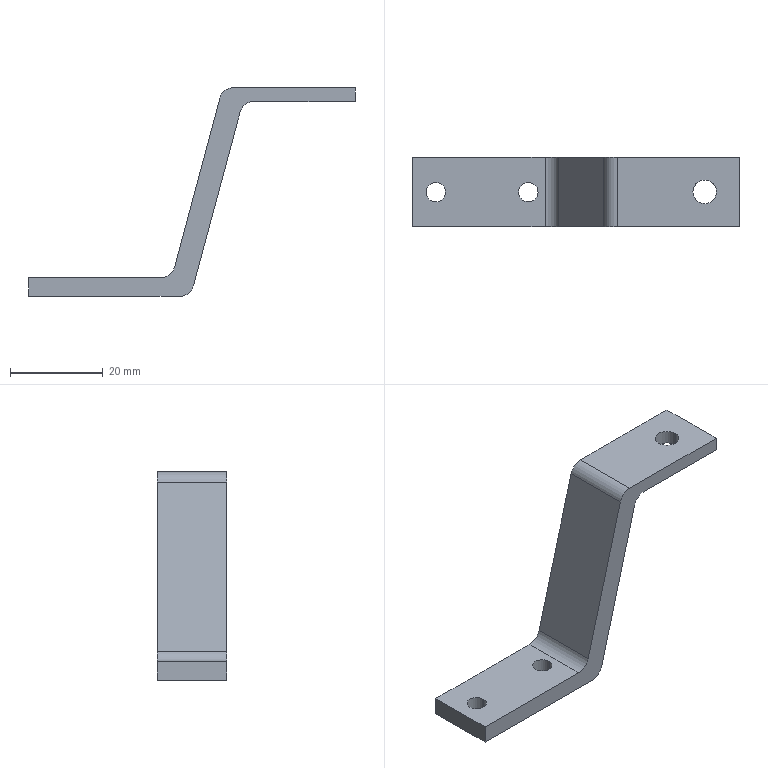Part | SolidWorks | features Extrusion 1, Fillet 1, ICE 1 | 1 solid | 20 faces | box 70.55 x 15 x 45 mm | volume 6219 mm3 | cylinder 10 | plane 10 | commonest cylinder face diameters 4.2 x4 6 x4 5.1 x2
STEP:
#1=CARTESIAN_POINT('',(27.1,7.5,4.));
#2=VERTEX_POINT('',#1);
#3=CARTESIAN_POINT('',(22.9,7.5,4.));
#4=VERTEX_POINT('',#3);
#5=CARTESIAN_POINT('',(25.,7.5,4.));
#6=DIRECTION('',(0.,0.,-1.));
#7=DIRECTION('',(-1.,0.,0.));
#8=AXIS2_PLACEMENT_3D('',#5,#6,#7);
#9=CIRCLE('',#8,2.1);
#10=EDGE_CURVE('',#2,#4,#9,.T.);
#11=ORIENTED_EDGE('',*,*,#10,.F.);
#12=CARTESIAN_POINT('',(27.1,7.5,0.));
#13=VERTEX_POINT('',#12);
#14=CARTESIAN_POINT('',(27.1,7.5,45.));
#15=DIRECTION('',(0.,0.,-1.));
#16=VECTOR('',#15,1000.);
#17=LINE('',#14,#16);
#18=EDGE_CURVE('',#2,#13,#17,.T.);
#19=ORIENTED_EDGE('',*,*,#18,.T.);
#20=CARTESIAN_POINT('',(22.9,7.5,0.));
#21=VERTEX_POINT('',#20);
#22=CARTESIAN_POINT('',(25.,7.5,0.));
#23=DIRECTION('',(0.,0.,-1.));
#24=DIRECTION('',(-1.,0.,0.));
#25=AXIS2_PLACEMENT_3D('',#22,#23,#24);
#26=CIRCLE('',#25,2.1);
#27=EDGE_CURVE('',#13,#21,#26,.T.);
#28=ORIENTED_EDGE('',*,*,#27,.T.);
#29=CARTESIAN_POINT('',(22.9,7.5,45.));
#30=DIRECTION('',(0.,0.,-1.));
#31=VECTOR('',#30,1000.);
#32=LINE('',#29,#31);
#33=EDGE_CURVE('',#4,#21,#32,.T.);
#34=ORIENTED_EDGE('',*,*,#33,.F.);
#35=EDGE_LOOP('',(#11,#19,#28,#34));
#36=FACE_OUTER_BOUND('',#35,.T.);
#37=CARTESIAN_POINT('',(25.,7.5,45.));
#38=DIRECTION('',(0.,0.,-1.));
#39=DIRECTION('',(-1.,0.,0.));
#40=AXIS2_PLACEMENT_3D('',#37,#38,#39);
#41=CYLINDRICAL_SURFACE('',#40,2.1);
#42=ADVANCED_FACE('',(#36),#41,.F.);
#43=CARTESIAN_POINT('',(7.1,7.5,4.));
#44=VERTEX_POINT('',#43);
#45=CARTESIAN_POINT('',(2.9,7.5,4.));
#46=VERTEX_POINT('',#45);
#47=CARTESIAN_POINT('',(5.,7.5,4.));
#48=DIRECTION('',(0.,0.,-1.));
#49=DIRECTION('',(-1.,0.,0.));
#50=AXIS2_PLACEMENT_3D('',#47,#48,#49);
#51=CIRCLE('',#50,2.1);
#52=EDGE_CURVE('',#44,#46,#51,.T.);
#53=ORIENTED_EDGE('',*,*,#52,.F.);
#54=CARTESIAN_POINT('',(7.1,7.5,0.));
#55=VERTEX_POINT('',#54);
#56=CARTESIAN_POINT('',(7.1,7.5,45.));
#57=DIRECTION('',(0.,0.,-1.));
#58=VECTOR('',#57,1000.);
#59=LINE('',#56,#58);
#60=EDGE_CURVE('',#44,#55,#59,.T.);
#61=ORIENTED_EDGE('',*,*,#60,.T.);
#62=CARTESIAN_POINT('',(2.9,7.5,0.));
#63=VERTEX_POINT('',#62);
#64=CARTESIAN_POINT('',(5.,7.5,0.));
#65=DIRECTION('',(0.,0.,-1.));
#66=DIRECTION('',(-1.,0.,0.));
#67=AXIS2_PLACEMENT_3D('',#64,#65,#66);
#68=CIRCLE('',#67,2.1);
#69=EDGE_CURVE('',#55,#63,#68,.T.);
#70=ORIENTED_EDGE('',*,*,#69,.T.);
#71=CARTESIAN_POINT('',(2.9,7.5,45.));
#72=DIRECTION('',(0.,0.,-1.));
#73=VECTOR('',#72,1000.);
#74=LINE('',#71,#73);
#75=EDGE_CURVE('',#46,#63,#74,.T.);
#76=ORIENTED_EDGE('',*,*,#75,.F.);
#77=EDGE_LOOP('',(#53,#61,#70,#76));
#78=FACE_OUTER_BOUND('',#77,.T.);
#79=CARTESIAN_POINT('',(5.,7.5,45.));
#80=DIRECTION('',(0.,0.,-1.));
#81=DIRECTION('',(-1.,0.,0.));
#82=AXIS2_PLACEMENT_3D('',#79,#80,#81);
#83=CYLINDRICAL_SURFACE('',#82,2.1);
#84=ADVANCED_FACE('',(#78),#83,.F.);
#85=CARTESIAN_POINT('',(65.6,7.5,45.));
#86=VERTEX_POINT('',#85);
#87=CARTESIAN_POINT('',(60.5,7.5,45.));
#88=VERTEX_POINT('',#87);
#89=CARTESIAN_POINT('',(63.05,7.5,45.));
#90=DIRECTION('',(0.,0.,-1.));
#91=DIRECTION('',(-1.,0.,0.));
#92=AXIS2_PLACEMENT_3D('',#89,#90,#91);
#93=CIRCLE('',#92,2.55);
#94=EDGE_CURVE('',#86,#88,#93,.T.);
#95=ORIENTED_EDGE('',*,*,#94,.F.);
#96=CARTESIAN_POINT('',(65.6,7.5,42.));
#97=VERTEX_POINT('',#96);
#98=CARTESIAN_POINT('',(65.6,7.5,45.));
#99=DIRECTION('',(0.,0.,-1.));
#100=VECTOR('',#99,1000.);
#101=LINE('',#98,#100);
#102=EDGE_CURVE('',#86,#97,#101,.T.);
#103=ORIENTED_EDGE('',*,*,#102,.T.);
#104=CARTESIAN_POINT('',(60.5,7.5,42.));
#105=VERTEX_POINT('',#104);
#106=CARTESIAN_POINT('',(63.05,7.5,42.));
#107=DIRECTION('',(0.,0.,1.));
#108=DIRECTION('',(1.,0.,0.));
#109=AXIS2_PLACEMENT_3D('',#106,#107,#108);
#110=CIRCLE('',#109,2.55);
#111=EDGE_CURVE('',#105,#97,#110,.T.);
#112=ORIENTED_EDGE('',*,*,#111,.F.);
#113=CARTESIAN_POINT('',(60.5,7.5,45.));
#114=DIRECTION('',(0.,0.,-1.));
#115=VECTOR('',#114,1000.);
#116=LINE('',#113,#115);
#117=EDGE_CURVE('',#88,#105,#116,.T.);
#118=ORIENTED_EDGE('',*,*,#117,.F.);
#119=EDGE_LOOP('',(#95,#103,#112,#118));
#120=FACE_OUTER_BOUND('',#119,.T.);
#121=CARTESIAN_POINT('',(63.05,7.5,45.));
#122=DIRECTION('',(0.,0.,-1.));
#123=DIRECTION('',(-1.,0.,0.));
#124=AXIS2_PLACEMENT_3D('',#121,#122,#123);
#125=CYLINDRICAL_SURFACE('',#124,2.55);
#126=ADVANCED_FACE('',(#120),#125,.F.);
#127=CARTESIAN_POINT('',(25.,7.5,0.));
#128=DIRECTION('',(0.,0.,-1.));
#129=DIRECTION('',(-1.,0.,0.));
#130=AXIS2_PLACEMENT_3D('',#127,#128,#129);
#131=CIRCLE('',#130,2.1);
#132=EDGE_CURVE('',#21,#13,#131,.T.);
#133=ORIENTED_EDGE('',*,*,#132,.F.);
#134=ORIENTED_EDGE('',*,*,#27,.F.);
#135=EDGE_LOOP('',(#133,#134));
#136=FACE_BOUND('',#135,.T.);
#137=CARTESIAN_POINT('',(5.,7.5,0.));
#138=DIRECTION('',(0.,0.,-1.));
#139=DIRECTION('',(-1.,0.,0.));
#140=AXIS2_PLACEMENT_3D('',#137,#138,#139);
#141=CIRCLE('',#140,2.1);
#142=EDGE_CURVE('',#63,#55,#141,.T.);
#143=ORIENTED_EDGE('',*,*,#142,.F.);
#144=ORIENTED_EDGE('',*,*,#69,.F.);
#145=EDGE_LOOP('',(#143,#144));
#146=FACE_BOUND('',#145,.T.);
#147=CARTESIAN_POINT('',(32.698,15.,0.));
#148=VERTEX_POINT('',#147);
#149=CARTESIAN_POINT('',(0.,15.,0.));
#150=VERTEX_POINT('',#149);
#151=CARTESIAN_POINT('',(35.,15.,0.));
#152=DIRECTION('',(-1.,0.,0.));
#153=VECTOR('',#152,1000.);
#154=LINE('',#151,#153);
#155=EDGE_CURVE('',#148,#150,#154,.T.);
#156=ORIENTED_EDGE('',*,*,#155,.F.);
#157=CARTESIAN_POINT('',(32.698,0.,0.));
#158=VERTEX_POINT('',#157);
#159=CARTESIAN_POINT('',(32.698,15.,0.));
#160=DIRECTION('',(0.,-1.,0.));
#161=VECTOR('',#160,1000.);
#162=LINE('',#159,#161);
#163=EDGE_CURVE('',#148,#158,#162,.T.);
#164=ORIENTED_EDGE('',*,*,#163,.T.);
#165=CARTESIAN_POINT('',(0.,0.,0.));
#166=VERTEX_POINT('',#165);
#167=CARTESIAN_POINT('',(35.,0.,0.));
#168=DIRECTION('',(-1.,0.,0.));
#169=VECTOR('',#168,1000.);
#170=LINE('',#167,#169);
#171=EDGE_CURVE('',#158,#166,#170,.T.);
#172=ORIENTED_EDGE('',*,*,#171,.T.);
#173=CARTESIAN_POINT('',(0.,15.,0.));
#174=DIRECTION('',(0.,-1.,0.));
#175=VECTOR('',#174,1000.);
#176=LINE('',#173,#175);
#177=EDGE_CURVE('',#150,#166,#176,.T.);
#178=ORIENTED_EDGE('',*,*,#177,.F.);
#179=EDGE_LOOP('',(#156,#164,#172,#178));
#180=FACE_OUTER_BOUND('',#179,.T.);
#181=CARTESIAN_POINT('',(35.,15.,0.));
#182=DIRECTION('',(0.,0.,1.));
#183=DIRECTION('',(1.,0.,0.));
#184=AXIS2_PLACEMENT_3D('',#181,#182,#183);
#185=PLANE('',#184);
#186=ADVANCED_FACE('',(#136,#146,#180),#185,.F.);
#187=CARTESIAN_POINT('',(0.,0.,4.));
#188=VERTEX_POINT('',#187);
#189=CARTESIAN_POINT('',(0.,0.,0.));
#190=DIRECTION('',(0.,0.,1.));
#191=VECTOR('',#190,1000.);
#192=LINE('',#189,#191);
#193=EDGE_CURVE('',#166,#188,#192,.T.);
#194=ORIENTED_EDGE('',*,*,#193,.T.);
#195=CARTESIAN_POINT('',(0.,15.,4.));
#196=VERTEX_POINT('',#195);
#197=CARTESIAN_POINT('',(0.,15.,4.));
#198=DIRECTION('',(0.,-1.,0.));
#199=VECTOR('',#198,1000.);
#200=LINE('',#197,#199);
#201=EDGE_CURVE('',#196,#188,#200,.T.);
#202=ORIENTED_EDGE('',*,*,#201,.F.);
#203=CARTESIAN_POINT('',(0.,15.,0.));
#204=DIRECTION('',(0.,0.,1.));
#205=VECTOR('',#204,1000.);
#206=LINE('',#203,#205);
#207=EDGE_CURVE('',#150,#196,#206,.T.);
#208=ORIENTED_EDGE('',*,*,#207,.F.);
#209=ORIENTED_EDGE('',*,*,#177,.T.);
#210=EDGE_LOOP('',(#194,#202,#208,#209));
#211=FACE_OUTER_BOUND('',#210,.T.);
#212=CARTESIAN_POINT('',(0.,15.,0.));
#213=DIRECTION('',(1.,0.,0.));
#214=DIRECTION('',(0.,0.,-1.));
#215=AXIS2_PLACEMENT_3D('',#212,#213,#214);
#216=PLANE('',#215);
#217=ADVANCED_FACE('',(#211),#216,.F.);
#218=CARTESIAN_POINT('',(25.,7.5,4.));
#219=DIRECTION('',(0.,0.,-1.));
#220=DIRECTION('',(-1.,0.,0.));
#221=AXIS2_PLACEMENT_3D('',#218,#219,#220);
#222=CIRCLE('',#221,2.1);
#223=EDGE_CURVE('',#4,#2,#222,.T.);
#224=ORIENTED_EDGE('',*,*,#223,.T.);
#225=ORIENTED_EDGE('',*,*,#10,.T.);
#226=EDGE_LOOP('',(#224,#225));
#227=FACE_BOUND('',#226,.T.);
#228=CARTESIAN_POINT('',(5.,7.5,4.));
#229=DIRECTION('',(0.,0.,-1.));
#230=DIRECTION('',(-1.,0.,0.));
#231=AXIS2_PLACEMENT_3D('',#228,#229,#230);
#232=CIRCLE('',#231,2.1);
#233=EDGE_CURVE('',#46,#44,#232,.T.);
#234=ORIENTED_EDGE('',*,*,#233,.T.);
#235=ORIENTED_EDGE('',*,*,#52,.T.);
#236=EDGE_LOOP('',(#234,#235));
#237=FACE_BOUND('',#236,.T.);
#238=CARTESIAN_POINT('',(28.593,0.,4.));
#239=VERTEX_POINT('',#238);
#240=CARTESIAN_POINT('',(0.,0.,4.));
#241=DIRECTION('',(1.,0.,0.));
#242=VECTOR('',#241,1000.);
#243=LINE('',#240,#242);
#244=EDGE_CURVE('',#188,#239,#243,.T.);
#245=ORIENTED_EDGE('',*,*,#244,.T.);
#246=CARTESIAN_POINT('',(28.593,15.,4.));
#247=VERTEX_POINT('',#246);
#248=CARTESIAN_POINT('',(28.593,15.,4.));
#249=DIRECTION('',(0.,1.,0.));
#250=VECTOR('',#249,1000.);
#251=LINE('',#248,#250);
#252=EDGE_CURVE('',#239,#247,#251,.T.);
#253=ORIENTED_EDGE('',*,*,#252,.T.);
#254=CARTESIAN_POINT('',(0.,15.,4.));
#255=DIRECTION('',(1.,0.,0.));
#256=VECTOR('',#255,1000.);
#257=LINE('',#254,#256);
#258=EDGE_CURVE('',#196,#247,#257,.T.);
#259=ORIENTED_EDGE('',*,*,#258,.F.);
#260=ORIENTED_EDGE('',*,*,#201,.T.);
#261=EDGE_LOOP('',(#245,#253,#259,#260));
#262=FACE_OUTER_BOUND('',#261,.T.);
#263=CARTESIAN_POINT('',(0.,15.,4.));
#264=DIRECTION('',(0.,0.,-1.));
#265=DIRECTION('',(-1.,0.,0.));
#266=AXIS2_PLACEMENT_3D('',#263,#264,#265);
#267=PLANE('',#266);
#268=ADVANCED_FACE('',(#227,#237,#262),#267,.F.);
#269=CARTESIAN_POINT('',(31.491,0.,6.224));
#270=VERTEX_POINT('',#269);
#271=CARTESIAN_POINT('',(41.286,0.,42.776));
#272=VERTEX_POINT('',#271);
#273=CARTESIAN_POINT('',(30.895,0.,4.));
#274=DIRECTION('',(0.2588,0.,0.9659));
#275=VECTOR('',#274,1000.);
#276=LINE('',#273,#275);
#277=EDGE_CURVE('',#270,#272,#276,.T.);
#278=ORIENTED_EDGE('',*,*,#277,.T.);
#279=CARTESIAN_POINT('',(41.286,15.,42.776));
#280=VERTEX_POINT('',#279);
#281=CARTESIAN_POINT('',(41.286,15.,42.776));
#282=DIRECTION('',(0.,1.,0.));
#283=VECTOR('',#282,1000.);
#284=LINE('',#281,#283);
#285=EDGE_CURVE('',#272,#280,#284,.T.);
#286=ORIENTED_EDGE('',*,*,#285,.T.);
#287=CARTESIAN_POINT('',(31.491,15.,6.224));
#288=VERTEX_POINT('',#287);
#289=CARTESIAN_POINT('',(30.895,15.,4.));
#290=DIRECTION('',(0.2588,0.,0.9659));
#291=VECTOR('',#290,1000.);
#292=LINE('',#289,#291);
#293=EDGE_CURVE('',#288,#280,#292,.T.);
#294=ORIENTED_EDGE('',*,*,#293,.F.);
#295=CARTESIAN_POINT('',(31.491,0.,6.224));
#296=DIRECTION('',(0.,-1.,0.));
#297=VECTOR('',#296,1000.);
#298=LINE('',#295,#297);
#299=EDGE_CURVE('',#288,#270,#298,.T.);
#300=ORIENTED_EDGE('',*,*,#299,.T.);
#301=EDGE_LOOP('',(#278,#286,#294,#300));
#302=FACE_OUTER_BOUND('',#301,.T.);
#303=CARTESIAN_POINT('',(30.895,15.,4.));
#304=DIRECTION('',(0.9659,0.,-0.2588));
#305=DIRECTION('',(-0.2588,0.,-0.9659));
#306=AXIS2_PLACEMENT_3D('',#303,#304,#305);
#307=PLANE('',#306);
#308=ADVANCED_FACE('',(#302),#307,.F.);
#309=CARTESIAN_POINT('',(63.05,7.5,45.));
#310=DIRECTION('',(0.,0.,-1.));
#311=DIRECTION('',(-1.,0.,0.));
#312=AXIS2_PLACEMENT_3D('',#309,#310,#311);
#313=CIRCLE('',#312,2.55);
#314=EDGE_CURVE('',#88,#86,#313,.T.);
#315=ORIENTED_EDGE('',*,*,#314,.T.);
#316=ORIENTED_EDGE('',*,*,#94,.T.);
#317=EDGE_LOOP('',(#315,#316));
#318=FACE_BOUND('',#317,.T.);
#319=CARTESIAN_POINT('',(44.183,15.,45.));
#320=VERTEX_POINT('',#319);
#321=CARTESIAN_POINT('',(70.55,15.,45.));
#322=VERTEX_POINT('',#321);
#323=CARTESIAN_POINT('',(41.881,15.,45.));
#324=DIRECTION('',(1.,0.,0.));
#325=VECTOR('',#324,1000.);
#326=LINE('',#323,#325);
#327=EDGE_CURVE('',#320,#322,#326,.T.);
#328=ORIENTED_EDGE('',*,*,#327,.F.);
#329=CARTESIAN_POINT('',(44.183,0.,45.));
#330=VERTEX_POINT('',#329);
#331=CARTESIAN_POINT('',(44.183,15.,45.));
#332=DIRECTION('',(0.,-1.,0.));
#333=VECTOR('',#332,1000.);
#334=LINE('',#331,#333);
#335=EDGE_CURVE('',#320,#330,#334,.T.);
#336=ORIENTED_EDGE('',*,*,#335,.T.);
#337=CARTESIAN_POINT('',(70.55,0.,45.));
#338=VERTEX_POINT('',#337);
#339=CARTESIAN_POINT('',(41.881,0.,45.));
#340=DIRECTION('',(1.,0.,0.));
#341=VECTOR('',#340,1000.);
#342=LINE('',#339,#341);
#343=EDGE_CURVE('',#330,#338,#342,.T.);
#344=ORIENTED_EDGE('',*,*,#343,.T.);
#345=CARTESIAN_POINT('',(70.55,15.,45.));
#346=DIRECTION('',(0.,-1.,0.));
#347=VECTOR('',#346,1000.);
#348=LINE('',#345,#347);
#349=EDGE_CURVE('',#322,#338,#348,.T.);
#350=ORIENTED_EDGE('',*,*,#349,.F.);
#351=EDGE_LOOP('',(#328,#336,#344,#350));
#352=FACE_OUTER_BOUND('',#351,.T.);
#353=CARTESIAN_POINT('',(41.881,15.,45.));
#354=DIRECTION('',(0.,0.,-1.));
#355=DIRECTION('',(-1.,0.,0.));
#356=AXIS2_PLACEMENT_3D('',#353,#354,#355);
#357=PLANE('',#356);
#358=ADVANCED_FACE('',(#318,#352),#357,.F.);
#359=CARTESIAN_POINT('',(70.55,0.,42.));
#360=VERTEX_POINT('',#359);
#361=CARTESIAN_POINT('',(70.55,0.,45.));
#362=DIRECTION('',(0.,0.,-1.));
#363=VECTOR('',#362,1000.);
#364=LINE('',#361,#363);
#365=EDGE_CURVE('',#338,#360,#364,.T.);
#366=ORIENTED_EDGE('',*,*,#365,.T.);
#367=CARTESIAN_POINT('',(70.55,15.,42.));
#368=VERTEX_POINT('',#367);
#369=CARTESIAN_POINT('',(70.55,15.,42.));
#370=DIRECTION('',(0.,-1.,0.));
#371=VECTOR('',#370,1000.);
#372=LINE('',#369,#371);
#373=EDGE_CURVE('',#368,#360,#372,.T.);
#374=ORIENTED_EDGE('',*,*,#373,.F.);
#375=CARTESIAN_POINT('',(70.55,15.,45.));
#376=DIRECTION('',(0.,0.,-1.));
#377=VECTOR('',#376,1000.);
#378=LINE('',#375,#377);
#379=EDGE_CURVE('',#322,#368,#378,.T.);
#380=ORIENTED_EDGE('',*,*,#379,.F.);
#381=ORIENTED_EDGE('',*,*,#349,.T.);
#382=EDGE_LOOP('',(#366,#374,#380,#381));
#383=FACE_OUTER_BOUND('',#382,.T.);
#384=CARTESIAN_POINT('',(70.55,15.,45.));
#385=DIRECTION('',(-1.,0.,0.));
#386=DIRECTION('',(0.,0.,1.));
#387=AXIS2_PLACEMENT_3D('',#384,#385,#386);
#388=PLANE('',#387);
#389=ADVANCED_FACE('',(#383),#388,.F.);
#390=ORIENTED_EDGE('',*,*,#111,.T.);
#391=CARTESIAN_POINT('',(63.05,7.5,42.));
#392=DIRECTION('',(0.,0.,1.));
#393=DIRECTION('',(1.,0.,0.));
#394=AXIS2_PLACEMENT_3D('',#391,#392,#393);
#395=CIRCLE('',#394,2.55);
#396=EDGE_CURVE('',#97,#105,#395,.T.);
#397=ORIENTED_EDGE('',*,*,#396,.T.);
#398=EDGE_LOOP('',(#390,#397));
#399=FACE_BOUND('',#398,.T.);
#400=CARTESIAN_POINT('',(48.556,0.,42.));
#401=VERTEX_POINT('',#400);
#402=CARTESIAN_POINT('',(70.55,0.,42.));
#403=DIRECTION('',(-1.,0.,0.));
#404=VECTOR('',#403,1000.);
#405=LINE('',#402,#404);
#406=EDGE_CURVE('',#360,#401,#405,.T.);
#407=ORIENTED_EDGE('',*,*,#406,.T.);
#408=CARTESIAN_POINT('',(48.556,15.,42.));
#409=VERTEX_POINT('',#408);
#410=CARTESIAN_POINT('',(48.556,15.,42.));
#411=DIRECTION('',(0.,1.,0.));
#412=VECTOR('',#411,1000.);
#413=LINE('',#410,#412);
#414=EDGE_CURVE('',#401,#409,#413,.T.);
#415=ORIENTED_EDGE('',*,*,#414,.T.);
#416=CARTESIAN_POINT('',(70.55,15.,42.));
#417=DIRECTION('',(-1.,0.,0.));
#418=VECTOR('',#417,1000.);
#419=LINE('',#416,#418);
#420=EDGE_CURVE('',#368,#409,#419,.T.);
#421=ORIENTED_EDGE('',*,*,#420,.F.);
#422=ORIENTED_EDGE('',*,*,#373,.T.);
#423=EDGE_LOOP('',(#407,#415,#421,#422));
#424=FACE_OUTER_BOUND('',#423,.T.);
#425=CARTESIAN_POINT('',(70.55,15.,42.));
#426=DIRECTION('',(0.,0.,1.));
#427=DIRECTION('',(1.,0.,0.));
#428=AXIS2_PLACEMENT_3D('',#425,#426,#427);
#429=PLANE('',#428);
#430=ADVANCED_FACE('',(#399,#424),#429,.F.);
#431=CARTESIAN_POINT('',(45.658,15.,39.776));
#432=VERTEX_POINT('',#431);
#433=CARTESIAN_POINT('',(35.596,15.,2.224));
#434=VERTEX_POINT('',#433);
#435=CARTESIAN_POINT('',(46.254,15.,42.));
#436=DIRECTION('',(-0.2588,0.,-0.9659));
#437=VECTOR('',#436,1000.);
#438=LINE('',#435,#437);
#439=EDGE_CURVE('',#432,#434,#438,.T.);
#440=ORIENTED_EDGE('',*,*,#439,.F.);
#441=CARTESIAN_POINT('',(45.658,0.,39.776));
#442=VERTEX_POINT('',#441);
#443=CARTESIAN_POINT('',(45.658,0.,39.776));
#444=DIRECTION('',(0.,-1.,0.));
#445=VECTOR('',#444,1000.);
#446=LINE('',#443,#445);
#447=EDGE_CURVE('',#432,#442,#446,.T.);
#448=ORIENTED_EDGE('',*,*,#447,.T.);
#449=CARTESIAN_POINT('',(35.596,0.,2.224));
#450=VERTEX_POINT('',#449);
#451=CARTESIAN_POINT('',(46.254,0.,42.));
#452=DIRECTION('',(-0.2588,0.,-0.9659));
#453=VECTOR('',#452,1000.);
#454=LINE('',#451,#453);
#455=EDGE_CURVE('',#442,#450,#454,.T.);
#456=ORIENTED_EDGE('',*,*,#455,.T.);
#457=CARTESIAN_POINT('',(35.596,15.,2.224));
#458=DIRECTION('',(0.,1.,0.));
#459=VECTOR('',#458,1000.);
#460=LINE('',#457,#459);
#461=EDGE_CURVE('',#450,#434,#460,.T.);
#462=ORIENTED_EDGE('',*,*,#461,.T.);
#463=EDGE_LOOP('',(#440,#448,#456,#462));
#464=FACE_OUTER_BOUND('',#463,.T.);
#465=CARTESIAN_POINT('',(46.254,15.,42.));
#466=DIRECTION('',(-0.9659,0.,0.2588));
#467=DIRECTION('',(0.2588,0.,0.9659));
#468=AXIS2_PLACEMENT_3D('',#465,#466,#467);
#469=PLANE('',#468);
#470=ADVANCED_FACE('',(#464),#469,.F.);
#471=ORIENTED_EDGE('',*,*,#293,.T.);
#472=CARTESIAN_POINT('',(44.183,15.,42.));
#473=DIRECTION('',(0.,1.,0.));
#474=DIRECTION('',(0.,0.,1.));
#475=AXIS2_PLACEMENT_3D('',#472,#473,#474);
#476=CIRCLE('',#475,3.);
#477=EDGE_CURVE('',#280,#320,#476,.T.);
#478=ORIENTED_EDGE('',*,*,#477,.T.);
#479=ORIENTED_EDGE('',*,*,#327,.T.);
#480=ORIENTED_EDGE('',*,*,#379,.T.);
#481=ORIENTED_EDGE('',*,*,#420,.T.);
#482=CARTESIAN_POINT('',(48.556,15.,39.));
#483=DIRECTION('',(0.,-1.,0.));
#484=DIRECTION('',(0.,0.,1.));
#485=AXIS2_PLACEMENT_3D('',#482,#483,#484);
#486=CIRCLE('',#485,3.);
#487=EDGE_CURVE('',#409,#432,#486,.T.);
#488=ORIENTED_EDGE('',*,*,#487,.T.);
#489=ORIENTED_EDGE('',*,*,#439,.T.);
#490=CARTESIAN_POINT('',(32.698,15.,3.));
#491=DIRECTION('',(0.,1.,0.));
#492=DIRECTION('',(0.,0.,1.));
#493=AXIS2_PLACEMENT_3D('',#490,#491,#492);
#494=CIRCLE('',#493,3.);
#495=EDGE_CURVE('',#434,#148,#494,.T.);
#496=ORIENTED_EDGE('',*,*,#495,.T.);
#497=ORIENTED_EDGE('',*,*,#155,.T.);
#498=ORIENTED_EDGE('',*,*,#207,.T.);
#499=ORIENTED_EDGE('',*,*,#258,.T.);
#500=CARTESIAN_POINT('',(28.593,15.,7.));
#501=DIRECTION('',(0.,-1.,0.));
#502=DIRECTION('',(0.,0.,1.));
#503=AXIS2_PLACEMENT_3D('',#500,#501,#502);
#504=CIRCLE('',#503,3.);
#505=EDGE_CURVE('',#247,#288,#504,.T.);
#506=ORIENTED_EDGE('',*,*,#505,.T.);
#507=EDGE_LOOP('',(#471,#478,#479,#480,#481,#488,#489,#496,#497,#498,#499,#506));
#508=FACE_OUTER_BOUND('',#507,.T.);
#509=CARTESIAN_POINT('',(0.,15.,0.));
#510=DIRECTION('',(0.,1.,0.));
#511=DIRECTION('',(0.,0.,1.));
#512=AXIS2_PLACEMENT_3D('',#509,#510,#511);
#513=PLANE('',#512);
#514=ADVANCED_FACE('',(#508),#513,.T.);
#515=ORIENTED_EDGE('',*,*,#343,.F.);
#516=CARTESIAN_POINT('',(44.183,0.,42.));
#517=DIRECTION('',(0.,-1.,0.));
#518=DIRECTION('',(0.,0.,1.));
#519=AXIS2_PLACEMENT_3D('',#516,#517,#518);
#520=CIRCLE('',#519,3.);
#521=EDGE_CURVE('',#330,#272,#520,.T.);
#522=ORIENTED_EDGE('',*,*,#521,.T.);
#523=ORIENTED_EDGE('',*,*,#277,.F.);
#524=CARTESIAN_POINT('',(28.593,0.,7.));
#525=DIRECTION('',(0.,1.,0.));
#526=DIRECTION('',(0.,0.,1.));
#527=AXIS2_PLACEMENT_3D('',#524,#525,#526);
#528=CIRCLE('',#527,3.);
#529=EDGE_CURVE('',#270,#239,#528,.T.);
#530=ORIENTED_EDGE('',*,*,#529,.T.);
#531=ORIENTED_EDGE('',*,*,#244,.F.);
#532=ORIENTED_EDGE('',*,*,#193,.F.);
#533=ORIENTED_EDGE('',*,*,#171,.F.);
#534=CARTESIAN_POINT('',(32.698,0.,3.));
#535=DIRECTION('',(0.,-1.,0.));
#536=DIRECTION('',(0.,0.,1.));
#537=AXIS2_PLACEMENT_3D('',#534,#535,#536);
#538=CIRCLE('',#537,3.);
#539=EDGE_CURVE('',#158,#450,#538,.T.);
#540=ORIENTED_EDGE('',*,*,#539,.T.);
#541=ORIENTED_EDGE('',*,*,#455,.F.);
#542=CARTESIAN_POINT('',(48.556,0.,39.));
#543=DIRECTION('',(0.,1.,0.));
#544=DIRECTION('',(0.,0.,1.));
#545=AXIS2_PLACEMENT_3D('',#542,#543,#544);
#546=CIRCLE('',#545,3.);
#547=EDGE_CURVE('',#442,#401,#546,.T.);
#548=ORIENTED_EDGE('',*,*,#547,.T.);
#549=ORIENTED_EDGE('',*,*,#406,.F.);
#550=ORIENTED_EDGE('',*,*,#365,.F.);
#551=EDGE_LOOP('',(#515,#522,#523,#530,#531,#532,#533,#540,#541,#548,#549,#550));
#552=FACE_OUTER_BOUND('',#551,.T.);
#553=CARTESIAN_POINT('',(0.,0.,0.));
#554=DIRECTION('',(0.,1.,0.));
#555=DIRECTION('',(0.,0.,1.));
#556=AXIS2_PLACEMENT_3D('',#553,#554,#555);
#557=PLANE('',#556);
#558=ADVANCED_FACE('',(#552),#557,.F.);
#559=ORIENTED_EDGE('',*,*,#102,.F.);
#560=ORIENTED_EDGE('',*,*,#314,.F.);
#561=ORIENTED_EDGE('',*,*,#117,.T.);
#562=ORIENTED_EDGE('',*,*,#396,.F.);
#563=EDGE_LOOP('',(#559,#560,#561,#562));
#564=FACE_OUTER_BOUND('',#563,.T.);
#565=CARTESIAN_POINT('',(63.05,7.5,45.));
#566=DIRECTION('',(0.,0.,-1.));
#567=DIRECTION('',(-1.,0.,0.));
#568=AXIS2_PLACEMENT_3D('',#565,#566,#567);
#569=CYLINDRICAL_SURFACE('',#568,2.55);
#570=ADVANCED_FACE('',(#564),#569,.F.);
#571=ORIENTED_EDGE('',*,*,#60,.F.);
#572=ORIENTED_EDGE('',*,*,#233,.F.);
#573=ORIENTED_EDGE('',*,*,#75,.T.);
#574=ORIENTED_EDGE('',*,*,#142,.T.);
#575=EDGE_LOOP('',(#571,#572,#573,#574));
#576=FACE_OUTER_BOUND('',#575,.T.);
#577=CARTESIAN_POINT('',(5.,7.5,45.));
#578=DIRECTION('',(0.,0.,-1.));
#579=DIRECTION('',(-1.,0.,0.));
#580=AXIS2_PLACEMENT_3D('',#577,#578,#579);
#581=CYLINDRICAL_SURFACE('',#580,2.1);
#582=ADVANCED_FACE('',(#576),#581,.F.);
#583=ORIENTED_EDGE('',*,*,#18,.F.);
#584=ORIENTED_EDGE('',*,*,#223,.F.);
#585=ORIENTED_EDGE('',*,*,#33,.T.);
#586=ORIENTED_EDGE('',*,*,#132,.T.);
#587=EDGE_LOOP('',(#583,#584,#585,#586));
#588=FACE_OUTER_BOUND('',#587,.T.);
#589=CARTESIAN_POINT('',(25.,7.5,45.));
#590=DIRECTION('',(0.,0.,-1.));
#591=DIRECTION('',(-1.,0.,0.));
#592=AXIS2_PLACEMENT_3D('',#589,#590,#591);
#593=CYLINDRICAL_SURFACE('',#592,2.1);
#594=ADVANCED_FACE('',(#588),#593,.F.);
#595=ORIENTED_EDGE('',*,*,#477,.F.);
#596=ORIENTED_EDGE('',*,*,#285,.F.);
#597=ORIENTED_EDGE('',*,*,#521,.F.);
#598=ORIENTED_EDGE('',*,*,#335,.F.);
#599=EDGE_LOOP('',(#595,#596,#597,#598));
#600=FACE_OUTER_BOUND('',#599,.T.);
#601=CARTESIAN_POINT('',(44.183,15.,42.));
#602=DIRECTION('',(0.,-1.,0.));
#603=DIRECTION('',(0.,0.,-1.));
#604=AXIS2_PLACEMENT_3D('',#601,#602,#603);
#605=CYLINDRICAL_SURFACE('',#604,3.);
#606=ADVANCED_FACE('',(#600),#605,.T.);
#607=ORIENTED_EDGE('',*,*,#487,.F.);
#608=ORIENTED_EDGE('',*,*,#414,.F.);
#609=ORIENTED_EDGE('',*,*,#547,.F.);
#610=ORIENTED_EDGE('',*,*,#447,.F.);
#611=EDGE_LOOP('',(#607,#608,#609,#610));
#612=FACE_OUTER_BOUND('',#611,.T.);
#613=CARTESIAN_POINT('',(48.556,15.,39.));
#614=DIRECTION('',(0.,1.,0.));
#615=DIRECTION('',(0.,0.,1.));
#616=AXIS2_PLACEMENT_3D('',#613,#614,#615);
#617=CYLINDRICAL_SURFACE('',#616,3.);
#618=ADVANCED_FACE('',(#612),#617,.F.);
#619=ORIENTED_EDGE('',*,*,#495,.F.);
#620=ORIENTED_EDGE('',*,*,#461,.F.);
#621=ORIENTED_EDGE('',*,*,#539,.F.);
#622=ORIENTED_EDGE('',*,*,#163,.F.);
#623=EDGE_LOOP('',(#619,#620,#621,#622));
#624=FACE_OUTER_BOUND('',#623,.T.);
#625=CARTESIAN_POINT('',(32.698,15.,3.));
#626=DIRECTION('',(0.,-1.,0.));
#627=DIRECTION('',(0.,0.,-1.));
#628=AXIS2_PLACEMENT_3D('',#625,#626,#627);
#629=CYLINDRICAL_SURFACE('',#628,3.);
#630=ADVANCED_FACE('',(#624),#629,.T.);
#631=ORIENTED_EDGE('',*,*,#505,.F.);
#632=ORIENTED_EDGE('',*,*,#252,.F.);
#633=ORIENTED_EDGE('',*,*,#529,.F.);
#634=ORIENTED_EDGE('',*,*,#299,.F.);
#635=EDGE_LOOP('',(#631,#632,#633,#634));
#636=FACE_OUTER_BOUND('',#635,.T.);
#637=CARTESIAN_POINT('',(28.593,15.,7.));
#638=DIRECTION('',(0.,1.,0.));
#639=DIRECTION('',(0.,0.,1.));
#640=AXIS2_PLACEMENT_3D('',#637,#638,#639);
#641=CYLINDRICAL_SURFACE('',#640,3.);
#642=ADVANCED_FACE('',(#636),#641,.F.);
#643=CLOSED_SHELL('',(#42,#84,#126,#186,#217,#268,#308,#358,#389,#430,#470,#514,#558,#570,#582,#594,#606,#618,#630,#642));
#644=MANIFOLD_SOLID_BREP('',#643);
#645=CARTESIAN_POINT('',(0.,0.,0.));
#646=DIRECTION('',(0.,0.,1.));
#647=DIRECTION('',(1.,0.,0.));
#648=AXIS2_PLACEMENT_3D('',#645,#646,#647);
#649=(LENGTH_UNIT()NAMED_UNIT(*)SI_UNIT(.MILLI.,.METRE.));
#650=UNCERTAINTY_MEASURE_WITH_UNIT(LENGTH_MEASURE(0.00001),#649,'','');
#651=(NAMED_UNIT(*)PLANE_ANGLE_UNIT()SI_UNIT($,.RADIAN.));
#652=(NAMED_UNIT(*)SI_UNIT($,.STERADIAN.)SOLID_ANGLE_UNIT());
#653=(GEOMETRIC_REPRESENTATION_CONTEXT(3)GLOBAL_UNCERTAINTY_ASSIGNED_CONTEXT((#650))GLOBAL_UNIT_ASSIGNED_CONTEXT((#649,#651,#652))REPRESENTATION_CONTEXT('',''));
#654=ADVANCED_BREP_SHAPE_REPRESENTATION('',(#644,#648),#653);